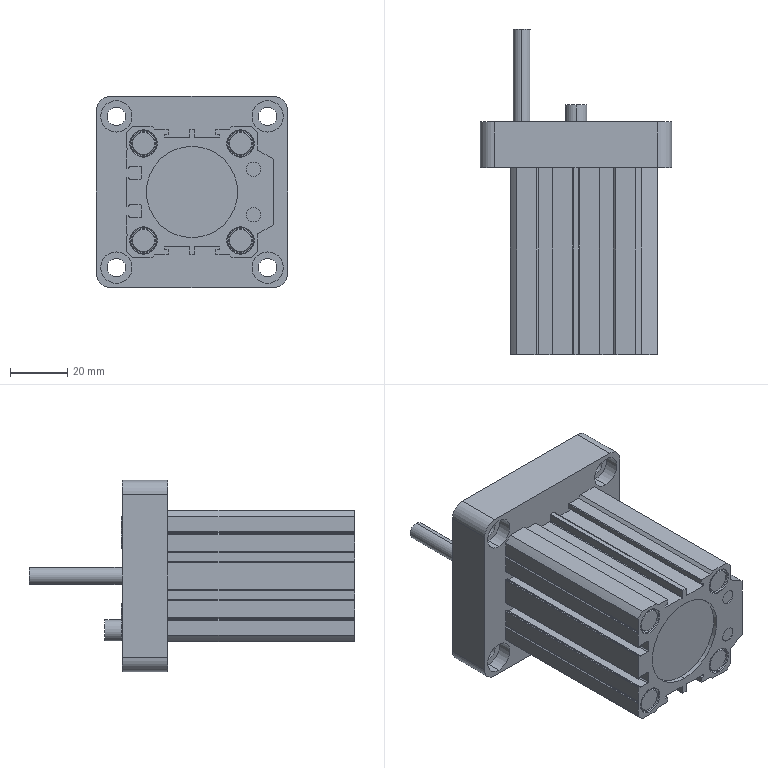Part | STEP file | TWH-S-32x20-K F-1-G _-0 | 1 solid | 256 faces | box 67 x 114 x 67 mm | volume 155824 mm3 | cylinder 130 | plane 102 | cone 24 | commonest cylinder face diameters 0.4 x34 6 x16 11 x16 0.8 x8 6.5 x8 8.4 x8